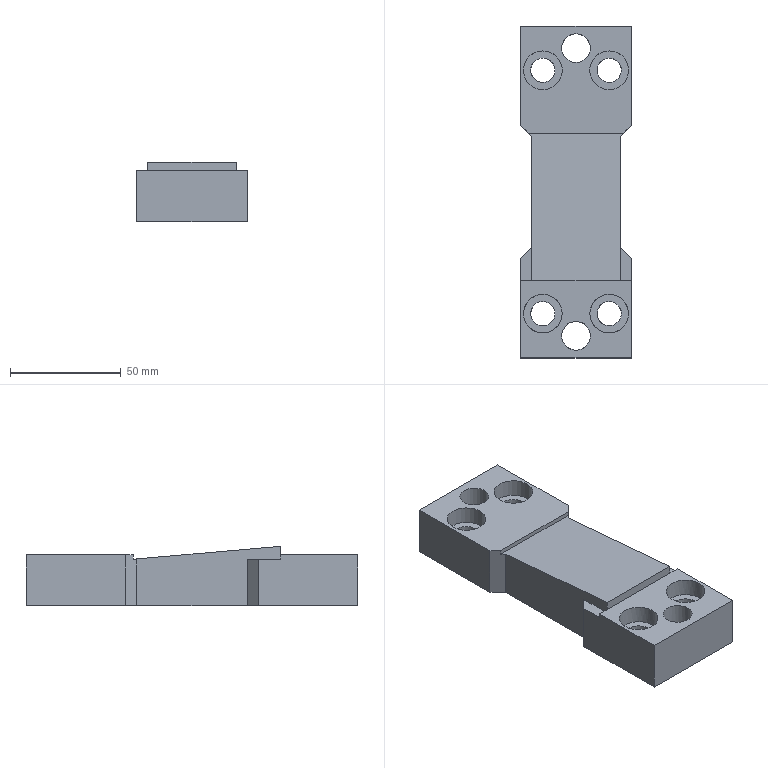Part | NX | features solid 2 | 1 solid | 36 faces | box 50 x 150 x 26.824 mm | volume 142519 mm3 | plane 26 | cylinder 10 | commonest cylinder face diameters 11 x4 17.5 x4 13 x2
STEP:
#1=CARTESIAN_POINT('',(-205.,-123.25,-57.));
#2=VERTEX_POINT('',#1);
#3=CARTESIAN_POINT('',(-205.,-132.,-57.));
#4=DIRECTION('',(0.,0.,1.));
#5=DIRECTION('',(0.,1.,0.));
#6=AXIS2_PLACEMENT_3D('',#3,#4,#5);
#7=CIRCLE('',#6,8.75);
#8=EDGE_CURVE('',#2,#2,#7,.T.);
#9=ORIENTED_EDGE('',*,*,#8,.F.);
#10=EDGE_LOOP('',(#9));
#11=FACE_BOUND('',#10,.T.);
#12=CARTESIAN_POINT('',(-220.,-115.5,-57.));
#13=VERTEX_POINT('',#12);
#14=CARTESIAN_POINT('',(-220.,-122.,-57.));
#15=DIRECTION('',(0.,0.,1.));
#16=DIRECTION('',(0.,1.,0.));
#17=AXIS2_PLACEMENT_3D('',#14,#15,#16);
#18=CIRCLE('',#17,6.5);
#19=EDGE_CURVE('',#13,#13,#18,.T.);
#20=ORIENTED_EDGE('',*,*,#19,.F.);
#21=EDGE_LOOP('',(#20));
#22=FACE_BOUND('',#21,.T.);
#23=CARTESIAN_POINT('',(-235.,-123.25,-57.));
#24=VERTEX_POINT('',#23);
#25=CARTESIAN_POINT('',(-235.,-132.,-57.));
#26=DIRECTION('',(0.,0.,1.));
#27=DIRECTION('',(0.,1.,0.));
#28=AXIS2_PLACEMENT_3D('',#25,#26,#27);
#29=CIRCLE('',#28,8.75);
#30=EDGE_CURVE('',#24,#24,#29,.T.);
#31=ORIENTED_EDGE('',*,*,#30,.F.);
#32=EDGE_LOOP('',(#31));
#33=FACE_BOUND('',#32,.T.);
#34=CARTESIAN_POINT('',(-241.57,-160.43,-57.));
#35=VERTEX_POINT('',#34);
#36=CARTESIAN_POINT('',(-198.43,-160.43,-57.));
#37=VERTEX_POINT('',#36);
#38=CARTESIAN_POINT('',(-240.,-160.43,-57.));
#39=DIRECTION('',(1.,0.,0.));
#40=VECTOR('',#39,1000.);
#41=LINE('',#38,#40);
#42=EDGE_CURVE('',#35,#37,#41,.T.);
#43=ORIENTED_EDGE('',*,*,#42,.T.);
#44=CARTESIAN_POINT('',(-195.,-157.,-57.));
#45=VERTEX_POINT('',#44);
#46=CARTESIAN_POINT('',(-200.,-162.,-57.));
#47=DIRECTION('',(0.7071,0.7071,0.));
#48=VECTOR('',#47,1000.);
#49=LINE('',#46,#48);
#50=EDGE_CURVE('',#37,#45,#49,.T.);
#51=ORIENTED_EDGE('',*,*,#50,.T.);
#52=CARTESIAN_POINT('',(-195.,-112.,-57.));
#53=VERTEX_POINT('',#52);
#54=CARTESIAN_POINT('',(-195.,-157.,-57.));
#55=DIRECTION('',(0.,1.,0.));
#56=VECTOR('',#55,1000.);
#57=LINE('',#54,#56);
#58=EDGE_CURVE('',#45,#53,#57,.T.);
#59=ORIENTED_EDGE('',*,*,#58,.T.);
#60=CARTESIAN_POINT('',(-245.,-112.,-57.));
#61=VERTEX_POINT('',#60);
#62=CARTESIAN_POINT('',(-245.,-112.,-57.));
#63=DIRECTION('',(1.,0.,0.));
#64=VECTOR('',#63,1000.);
#65=LINE('',#62,#64);
#66=EDGE_CURVE('',#61,#53,#65,.T.);
#67=ORIENTED_EDGE('',*,*,#66,.F.);
#68=CARTESIAN_POINT('',(-245.,-157.,-57.));
#69=VERTEX_POINT('',#68);
#70=CARTESIAN_POINT('',(-245.,-157.,-57.));
#71=DIRECTION('',(0.,1.,0.));
#72=VECTOR('',#71,1000.);
#73=LINE('',#70,#72);
#74=EDGE_CURVE('',#69,#61,#73,.T.);
#75=ORIENTED_EDGE('',*,*,#74,.F.);
#76=CARTESIAN_POINT('',(-240.,-162.,-57.));
#77=DIRECTION('',(-0.7071,0.7071,0.));
#78=VECTOR('',#77,1000.);
#79=LINE('',#76,#78);
#80=EDGE_CURVE('',#35,#69,#79,.T.);
#81=ORIENTED_EDGE('',*,*,#80,.F.);
#82=EDGE_LOOP('',(#43,#51,#59,#67,#75,#81));
#83=FACE_BOUND('',#82,.T.);
#84=CARTESIAN_POINT('',(-245.,-262.,-57.));
#85=DIRECTION('',(0.,0.,-1.));
#86=DIRECTION('',(-1.,0.,0.));
#87=AXIS2_PLACEMENT_3D('',#84,#85,#86);
#88=PLANE('',#87);
#89=ADVANCED_FACE('',(#11,#22,#33,#83),#88,.F.);
#90=CARTESIAN_POINT('',(-200.,-162.,-58.863));
#91=VERTEX_POINT('',#90);
#92=CARTESIAN_POINT('',(-200.,-162.,-80.));
#93=VERTEX_POINT('',#92);
#94=CARTESIAN_POINT('',(-200.,-162.,-59.));
#95=DIRECTION('',(0.,0.,-1.));
#96=VECTOR('',#95,1000.);
#97=LINE('',#94,#96);
#98=EDGE_CURVE('',#91,#93,#97,.T.);
#99=ORIENTED_EDGE('',*,*,#98,.F.);
#100=CARTESIAN_POINT('',(-200.,-227.,-53.176));
#101=VERTEX_POINT('',#100);
#102=CARTESIAN_POINT('',(-200.,-227.,-53.176));
#103=DIRECTION('',(0.,0.9962,-0.08716));
#104=VECTOR('',#103,1000.);
#105=LINE('',#102,#104);
#106=EDGE_CURVE('',#101,#91,#105,.T.);
#107=ORIENTED_EDGE('',*,*,#106,.F.);
#108=CARTESIAN_POINT('',(-200.,-227.,-57.));
#109=VERTEX_POINT('',#108);
#110=CARTESIAN_POINT('',(-200.,-227.,-53.176));
#111=DIRECTION('',(0.,0.,-1.));
#112=VECTOR('',#111,1000.);
#113=LINE('',#110,#112);
#114=EDGE_CURVE('',#101,#109,#113,.T.);
#115=ORIENTED_EDGE('',*,*,#114,.T.);
#116=CARTESIAN_POINT('',(-200.,-227.,-59.));
#117=VERTEX_POINT('',#116);
#118=CARTESIAN_POINT('',(-200.,-227.,-53.176));
#119=DIRECTION('',(0.,0.,-1.));
#120=VECTOR('',#119,1000.);
#121=LINE('',#118,#120);
#122=EDGE_CURVE('',#109,#117,#121,.T.);
#123=ORIENTED_EDGE('',*,*,#122,.T.);
#124=CARTESIAN_POINT('',(-200.,-212.,-59.));
#125=VERTEX_POINT('',#124);
#126=CARTESIAN_POINT('',(-200.,-160.43,-59.));
#127=DIRECTION('',(0.,-1.,0.));
#128=VECTOR('',#127,1000.);
#129=LINE('',#126,#128);
#130=EDGE_CURVE('',#125,#117,#129,.T.);
#131=ORIENTED_EDGE('',*,*,#130,.F.);
#132=CARTESIAN_POINT('',(-200.,-212.,-80.));
#133=VERTEX_POINT('',#132);
#134=CARTESIAN_POINT('',(-200.,-212.,-59.));
#135=DIRECTION('',(0.,0.,-1.));
#136=VECTOR('',#135,1000.);
#137=LINE('',#134,#136);
#138=EDGE_CURVE('',#125,#133,#137,.T.);
#139=ORIENTED_EDGE('',*,*,#138,.T.);
#140=CARTESIAN_POINT('',(-200.,-212.,-80.));
#141=DIRECTION('',(0.,1.,0.));
#142=VECTOR('',#141,1000.);
#143=LINE('',#140,#142);
#144=EDGE_CURVE('',#133,#93,#143,.T.);
#145=ORIENTED_EDGE('',*,*,#144,.T.);
#146=EDGE_LOOP('',(#99,#107,#115,#123,#131,#139,#145));
#147=FACE_BOUND('',#146,.T.);
#148=CARTESIAN_POINT('',(-200.,-212.,-59.));
#149=DIRECTION('',(-1.,0.,0.));
#150=DIRECTION('',(0.,-1.,0.));
#151=AXIS2_PLACEMENT_3D('',#148,#149,#150);
#152=PLANE('',#151);
#153=ADVANCED_FACE('',(#147),#152,.F.);
#154=CARTESIAN_POINT('',(-240.,-227.,-53.176));
#155=VERTEX_POINT('',#154);
#156=CARTESIAN_POINT('',(-240.,-227.,-57.));
#157=VERTEX_POINT('',#156);
#158=CARTESIAN_POINT('',(-240.,-227.,-53.176));
#159=DIRECTION('',(0.,0.,-1.));
#160=VECTOR('',#159,1000.);
#161=LINE('',#158,#160);
#162=EDGE_CURVE('',#155,#157,#161,.T.);
#163=ORIENTED_EDGE('',*,*,#162,.T.);
#164=CARTESIAN_POINT('',(-240.,-227.,-57.));
#165=DIRECTION('',(1.,0.,0.));
#166=VECTOR('',#165,1000.);
#167=LINE('',#164,#166);
#168=EDGE_CURVE('',#157,#109,#167,.T.);
#169=ORIENTED_EDGE('',*,*,#168,.T.);
#170=ORIENTED_EDGE('',*,*,#114,.F.);
#171=CARTESIAN_POINT('',(-240.,-227.,-53.176));
#172=DIRECTION('',(1.,0.,0.));
#173=VECTOR('',#172,1000.);
#174=LINE('',#171,#173);
#175=EDGE_CURVE('',#155,#101,#174,.T.);
#176=ORIENTED_EDGE('',*,*,#175,.F.);
#177=EDGE_LOOP('',(#163,#169,#170,#176));
#178=FACE_BOUND('',#177,.T.);
#179=CARTESIAN_POINT('',(-240.,-227.,-53.176));
#180=DIRECTION('',(0.,-1.,0.));
#181=DIRECTION('',(1.,0.,0.));
#182=AXIS2_PLACEMENT_3D('',#179,#180,#181);
#183=PLANE('',#182);
#184=ADVANCED_FACE('',(#178),#183,.T.);
#185=ORIENTED_EDGE('',*,*,#130,.T.);
#186=CARTESIAN_POINT('',(-195.,-227.,-59.));
#187=VERTEX_POINT('',#186);
#188=CARTESIAN_POINT('',(-245.,-227.,-59.));
#189=DIRECTION('',(1.,0.,0.));
#190=VECTOR('',#189,1000.);
#191=LINE('',#188,#190);
#192=EDGE_CURVE('',#117,#187,#191,.T.);
#193=ORIENTED_EDGE('',*,*,#192,.T.);
#194=CARTESIAN_POINT('',(-195.,-217.,-59.));
#195=VERTEX_POINT('',#194);
#196=CARTESIAN_POINT('',(-195.,-262.,-59.));
#197=DIRECTION('',(0.,1.,0.));
#198=VECTOR('',#197,1000.);
#199=LINE('',#196,#198);
#200=EDGE_CURVE('',#187,#195,#199,.T.);
#201=ORIENTED_EDGE('',*,*,#200,.T.);
#202=CARTESIAN_POINT('',(-200.,-212.,-59.));
#203=DIRECTION('',(0.7071,-0.7071,0.));
#204=VECTOR('',#203,1000.);
#205=LINE('',#202,#204);
#206=EDGE_CURVE('',#125,#195,#205,.T.);
#207=ORIENTED_EDGE('',*,*,#206,.F.);
#208=EDGE_LOOP('',(#185,#193,#201,#207));
#209=FACE_BOUND('',#208,.T.);
#210=CARTESIAN_POINT('',(-245.,-262.,-59.));
#211=DIRECTION('',(0.,0.,-1.));
#212=DIRECTION('',(-1.,0.,0.));
#213=AXIS2_PLACEMENT_3D('',#210,#211,#212);
#214=PLANE('',#213);
#215=ADVANCED_FACE('',(#209),#214,.F.);
#216=CARTESIAN_POINT('',(-245.,-227.,-59.));
#217=VERTEX_POINT('',#216);
#218=CARTESIAN_POINT('',(-240.,-227.,-59.));
#219=VERTEX_POINT('',#218);
#220=CARTESIAN_POINT('',(-245.,-227.,-59.));
#221=DIRECTION('',(1.,0.,0.));
#222=VECTOR('',#221,1000.);
#223=LINE('',#220,#222);
#224=EDGE_CURVE('',#217,#219,#223,.T.);
#225=ORIENTED_EDGE('',*,*,#224,.T.);
#226=CARTESIAN_POINT('',(-240.,-212.,-59.));
#227=VERTEX_POINT('',#226);
#228=CARTESIAN_POINT('',(-240.,-160.43,-59.));
#229=DIRECTION('',(0.,-1.,0.));
#230=VECTOR('',#229,1000.);
#231=LINE('',#228,#230);
#232=EDGE_CURVE('',#227,#219,#231,.T.);
#233=ORIENTED_EDGE('',*,*,#232,.F.);
#234=CARTESIAN_POINT('',(-245.,-217.,-59.));
#235=VERTEX_POINT('',#234);
#236=CARTESIAN_POINT('',(-245.,-217.,-59.));
#237=DIRECTION('',(0.7071,0.7071,0.));
#238=VECTOR('',#237,1000.);
#239=LINE('',#236,#238);
#240=EDGE_CURVE('',#235,#227,#239,.T.);
#241=ORIENTED_EDGE('',*,*,#240,.F.);
#242=CARTESIAN_POINT('',(-245.,-262.,-59.));
#243=DIRECTION('',(0.,1.,0.));
#244=VECTOR('',#243,1000.);
#245=LINE('',#242,#244);
#246=EDGE_CURVE('',#217,#235,#245,.T.);
#247=ORIENTED_EDGE('',*,*,#246,.F.);
#248=EDGE_LOOP('',(#225,#233,#241,#247));
#249=FACE_BOUND('',#248,.T.);
#250=CARTESIAN_POINT('',(-245.,-262.,-59.));
#251=DIRECTION('',(0.,0.,-1.));
#252=DIRECTION('',(-1.,0.,0.));
#253=AXIS2_PLACEMENT_3D('',#250,#251,#252);
#254=PLANE('',#253);
#255=ADVANCED_FACE('',(#249),#254,.F.);
#256=ORIENTED_EDGE('',*,*,#192,.F.);
#257=ORIENTED_EDGE('',*,*,#122,.F.);
#258=CARTESIAN_POINT('',(-195.,-227.,-57.));
#259=VERTEX_POINT('',#258);
#260=CARTESIAN_POINT('',(-245.,-227.,-57.));
#261=DIRECTION('',(1.,0.,0.));
#262=VECTOR('',#261,1000.);
#263=LINE('',#260,#262);
#264=EDGE_CURVE('',#109,#259,#263,.T.);
#265=ORIENTED_EDGE('',*,*,#264,.T.);
#266=CARTESIAN_POINT('',(-195.,-227.,-59.));
#267=DIRECTION('',(0.,0.,-1.));
#268=VECTOR('',#267,1000.);
#269=LINE('',#266,#268);
#270=EDGE_CURVE('',#259,#187,#269,.T.);
#271=ORIENTED_EDGE('',*,*,#270,.T.);
#272=EDGE_LOOP('',(#256,#257,#265,#271));
#273=FACE_BOUND('',#272,.T.);
#274=CARTESIAN_POINT('',(-245.,-227.,-40.44));
#275=DIRECTION('',(0.,1.,0.));
#276=DIRECTION('',(-1.,0.,0.));
#277=AXIS2_PLACEMENT_3D('',#274,#275,#276);
#278=PLANE('',#277);
#279=ADVANCED_FACE('',(#273),#278,.T.);
#280=CARTESIAN_POINT('',(-205.,-126.5,-80.));
#281=VERTEX_POINT('',#280);
#282=CARTESIAN_POINT('',(-205.,-132.,-80.));
#283=DIRECTION('',(0.,0.,1.));
#284=DIRECTION('',(0.,1.,0.));
#285=AXIS2_PLACEMENT_3D('',#282,#283,#284);
#286=CIRCLE('',#285,5.5);
#287=EDGE_CURVE('',#281,#281,#286,.T.);
#288=ORIENTED_EDGE('',*,*,#287,.F.);
#289=EDGE_LOOP('',(#288));
#290=FACE_BOUND('',#289,.T.);
#291=CARTESIAN_POINT('',(-199.5,-132.,-65.));
#292=VERTEX_POINT('',#291);
#293=CARTESIAN_POINT('',(-205.,-132.,-65.));
#294=DIRECTION('',(0.,0.,1.));
#295=DIRECTION('',(1.,0.,0.));
#296=AXIS2_PLACEMENT_3D('',#293,#294,#295);
#297=CIRCLE('',#296,5.5);
#298=EDGE_CURVE('',#292,#292,#297,.T.);
#299=ORIENTED_EDGE('',*,*,#298,.T.);
#300=EDGE_LOOP('',(#299));
#301=FACE_BOUND('',#300,.T.);
#302=CARTESIAN_POINT('',(-205.,-132.,-59.));
#303=DIRECTION('',(0.,0.,-1.));
#304=DIRECTION('',(-1.,0.,0.));
#305=AXIS2_PLACEMENT_3D('',#302,#303,#304);
#306=CYLINDRICAL_SURFACE('',#305,5.5);
#307=ADVANCED_FACE('',(#290,#301),#306,.F.);
#308=CARTESIAN_POINT('',(-235.,-126.5,-80.));
#309=VERTEX_POINT('',#308);
#310=CARTESIAN_POINT('',(-235.,-132.,-80.));
#311=DIRECTION('',(0.,0.,1.));
#312=DIRECTION('',(0.,1.,0.));
#313=AXIS2_PLACEMENT_3D('',#310,#311,#312);
#314=CIRCLE('',#313,5.5);
#315=EDGE_CURVE('',#309,#309,#314,.T.);
#316=ORIENTED_EDGE('',*,*,#315,.F.);
#317=EDGE_LOOP('',(#316));
#318=FACE_BOUND('',#317,.T.);
#319=CARTESIAN_POINT('',(-229.5,-132.,-65.));
#320=VERTEX_POINT('',#319);
#321=CARTESIAN_POINT('',(-235.,-132.,-65.));
#322=DIRECTION('',(0.,0.,1.));
#323=DIRECTION('',(1.,0.,0.));
#324=AXIS2_PLACEMENT_3D('',#321,#322,#323);
#325=CIRCLE('',#324,5.5);
#326=EDGE_CURVE('',#320,#320,#325,.T.);
#327=ORIENTED_EDGE('',*,*,#326,.T.);
#328=EDGE_LOOP('',(#327));
#329=FACE_BOUND('',#328,.T.);
#330=CARTESIAN_POINT('',(-235.,-132.,-59.));
#331=DIRECTION('',(0.,0.,-1.));
#332=DIRECTION('',(-1.,0.,0.));
#333=AXIS2_PLACEMENT_3D('',#330,#331,#332);
#334=CYLINDRICAL_SURFACE('',#333,5.5);
#335=ADVANCED_FACE('',(#318,#329),#334,.F.);
#336=CARTESIAN_POINT('',(-195.,-262.,-80.));
#337=VERTEX_POINT('',#336);
#338=CARTESIAN_POINT('',(-195.,-217.,-80.));
#339=VERTEX_POINT('',#338);
#340=CARTESIAN_POINT('',(-195.,-262.,-80.));
#341=DIRECTION('',(0.,1.,0.));
#342=VECTOR('',#341,1000.);
#343=LINE('',#340,#342);
#344=EDGE_CURVE('',#337,#339,#343,.T.);
#345=ORIENTED_EDGE('',*,*,#344,.F.);
#346=CARTESIAN_POINT('',(-245.,-262.,-80.));
#347=VERTEX_POINT('',#346);
#348=CARTESIAN_POINT('',(-195.,-262.,-80.));
#349=DIRECTION('',(-1.,0.,0.));
#350=VECTOR('',#349,1000.);
#351=LINE('',#348,#350);
#352=EDGE_CURVE('',#337,#347,#351,.T.);
#353=ORIENTED_EDGE('',*,*,#352,.T.);
#354=CARTESIAN_POINT('',(-245.,-217.,-80.));
#355=VERTEX_POINT('',#354);
#356=CARTESIAN_POINT('',(-245.,-262.,-80.));
#357=DIRECTION('',(0.,1.,0.));
#358=VECTOR('',#357,1000.);
#359=LINE('',#356,#358);
#360=EDGE_CURVE('',#347,#355,#359,.T.);
#361=ORIENTED_EDGE('',*,*,#360,.T.);
#362=CARTESIAN_POINT('',(-240.,-212.,-80.));
#363=VERTEX_POINT('',#362);
#364=CARTESIAN_POINT('',(-245.,-217.,-80.));
#365=DIRECTION('',(0.7071,0.7071,0.));
#366=VECTOR('',#365,1000.);
#367=LINE('',#364,#366);
#368=EDGE_CURVE('',#355,#363,#367,.T.);
#369=ORIENTED_EDGE('',*,*,#368,.T.);
#370=CARTESIAN_POINT('',(-240.,-162.,-80.));
#371=VERTEX_POINT('',#370);
#372=CARTESIAN_POINT('',(-240.,-212.,-80.));
#373=DIRECTION('',(0.,1.,0.));
#374=VECTOR('',#373,1000.);
#375=LINE('',#372,#374);
#376=EDGE_CURVE('',#363,#371,#375,.T.);
#377=ORIENTED_EDGE('',*,*,#376,.T.);
#378=CARTESIAN_POINT('',(-245.,-157.,-80.));
#379=VERTEX_POINT('',#378);
#380=CARTESIAN_POINT('',(-240.,-162.,-80.));
#381=DIRECTION('',(-0.7071,0.7071,0.));
#382=VECTOR('',#381,1000.);
#383=LINE('',#380,#382);
#384=EDGE_CURVE('',#371,#379,#383,.T.);
#385=ORIENTED_EDGE('',*,*,#384,.T.);
#386=CARTESIAN_POINT('',(-245.,-112.,-80.));
#387=VERTEX_POINT('',#386);
#388=CARTESIAN_POINT('',(-245.,-157.,-80.));
#389=DIRECTION('',(0.,1.,0.));
#390=VECTOR('',#389,1000.);
#391=LINE('',#388,#390);
#392=EDGE_CURVE('',#379,#387,#391,.T.);
#393=ORIENTED_EDGE('',*,*,#392,.T.);
#394=CARTESIAN_POINT('',(-195.,-112.,-80.));
#395=VERTEX_POINT('',#394);
#396=CARTESIAN_POINT('',(-245.,-112.,-80.));
#397=DIRECTION('',(1.,0.,0.));
#398=VECTOR('',#397,1000.);
#399=LINE('',#396,#398);
#400=EDGE_CURVE('',#387,#395,#399,.T.);
#401=ORIENTED_EDGE('',*,*,#400,.T.);
#402=CARTESIAN_POINT('',(-195.,-157.,-80.));
#403=VERTEX_POINT('',#402);
#404=CARTESIAN_POINT('',(-195.,-157.,-80.));
#405=DIRECTION('',(0.,1.,0.));
#406=VECTOR('',#405,1000.);
#407=LINE('',#404,#406);
#408=EDGE_CURVE('',#403,#395,#407,.T.);
#409=ORIENTED_EDGE('',*,*,#408,.F.);
#410=CARTESIAN_POINT('',(-200.,-162.,-80.));
#411=DIRECTION('',(0.7071,0.7071,0.));
#412=VECTOR('',#411,1000.);
#413=LINE('',#410,#412);
#414=EDGE_CURVE('',#93,#403,#413,.T.);
#415=ORIENTED_EDGE('',*,*,#414,.F.);
#416=ORIENTED_EDGE('',*,*,#144,.F.);
#417=CARTESIAN_POINT('',(-200.,-212.,-80.));
#418=DIRECTION('',(0.7071,-0.7071,0.));
#419=VECTOR('',#418,1000.);
#420=LINE('',#417,#419);
#421=EDGE_CURVE('',#133,#339,#420,.T.);
#422=ORIENTED_EDGE('',*,*,#421,.T.);
#423=EDGE_LOOP('',(#345,#353,#361,#369,#377,#385,#393,#401,#409,#415,#416,#422));
#424=FACE_BOUND('',#423,.T.);
#425=ORIENTED_EDGE('',*,*,#287,.T.);
#426=EDGE_LOOP('',(#425));
#427=FACE_BOUND('',#426,.T.);
#428=ORIENTED_EDGE('',*,*,#315,.T.);
#429=EDGE_LOOP('',(#428));
#430=FACE_BOUND('',#429,.T.);
#431=CARTESIAN_POINT('',(-220.,-115.5,-80.));
#432=VERTEX_POINT('',#431);
#433=CARTESIAN_POINT('',(-220.,-122.,-80.));
#434=DIRECTION('',(0.,0.,1.));
#435=DIRECTION('',(0.,1.,0.));
#436=AXIS2_PLACEMENT_3D('',#433,#434,#435);
#437=CIRCLE('',#436,6.5);
#438=EDGE_CURVE('',#432,#432,#437,.T.);
#439=ORIENTED_EDGE('',*,*,#438,.T.);
#440=EDGE_LOOP('',(#439));
#441=FACE_BOUND('',#440,.T.);
#442=CARTESIAN_POINT('',(-205.,-236.5,-80.));
#443=VERTEX_POINT('',#442);
#444=CARTESIAN_POINT('',(-205.,-242.,-80.));
#445=DIRECTION('',(0.,0.,1.));
#446=DIRECTION('',(0.,1.,0.));
#447=AXIS2_PLACEMENT_3D('',#444,#445,#446);
#448=CIRCLE('',#447,5.5);
#449=EDGE_CURVE('',#443,#443,#448,.T.);
#450=ORIENTED_EDGE('',*,*,#449,.T.);
#451=EDGE_LOOP('',(#450));
#452=FACE_BOUND('',#451,.T.);
#453=CARTESIAN_POINT('',(-235.,-236.5,-80.));
#454=VERTEX_POINT('',#453);
#455=CARTESIAN_POINT('',(-235.,-242.,-80.));
#456=DIRECTION('',(0.,0.,1.));
#457=DIRECTION('',(0.,1.,0.));
#458=AXIS2_PLACEMENT_3D('',#455,#456,#457);
#459=CIRCLE('',#458,5.5);
#460=EDGE_CURVE('',#454,#454,#459,.T.);
#461=ORIENTED_EDGE('',*,*,#460,.T.);
#462=EDGE_LOOP('',(#461));
#463=FACE_BOUND('',#462,.T.);
#464=CARTESIAN_POINT('',(-220.,-245.5,-80.));
#465=VERTEX_POINT('',#464);
#466=CARTESIAN_POINT('',(-220.,-252.,-80.));
#467=DIRECTION('',(0.,0.,1.));
#468=DIRECTION('',(0.,1.,0.));
#469=AXIS2_PLACEMENT_3D('',#466,#467,#468);
#470=CIRCLE('',#469,6.5);
#471=EDGE_CURVE('',#465,#465,#470,.T.);
#472=ORIENTED_EDGE('',*,*,#471,.T.);
#473=EDGE_LOOP('',(#472));
#474=FACE_BOUND('',#473,.T.);
#475=CARTESIAN_POINT('',(-245.,-262.,-80.));
#476=DIRECTION('',(0.,0.,-1.));
#477=DIRECTION('',(-1.,0.,0.));
#478=AXIS2_PLACEMENT_3D('',#475,#476,#477);
#479=PLANE('',#478);
#480=ADVANCED_FACE('',(#424,#427,#430,#441,#452,#463,#474),#479,.T.);
#481=ORIENTED_EDGE('',*,*,#360,.F.);
#482=CARTESIAN_POINT('',(-245.,-262.,-57.));
#483=VERTEX_POINT('',#482);
#484=CARTESIAN_POINT('',(-245.,-262.,-59.));
#485=DIRECTION('',(0.,0.,-1.));
#486=VECTOR('',#485,1000.);
#487=LINE('',#484,#486);
#488=EDGE_CURVE('',#483,#347,#487,.T.);
#489=ORIENTED_EDGE('',*,*,#488,.F.);
#490=CARTESIAN_POINT('',(-245.,-227.,-57.));
#491=VERTEX_POINT('',#490);
#492=CARTESIAN_POINT('',(-245.,-262.,-57.));
#493=DIRECTION('',(0.,1.,0.));
#494=VECTOR('',#493,1000.);
#495=LINE('',#492,#494);
#496=EDGE_CURVE('',#483,#491,#495,.T.);
#497=ORIENTED_EDGE('',*,*,#496,.T.);
#498=CARTESIAN_POINT('',(-245.,-227.,-59.));
#499=DIRECTION('',(0.,0.,-1.));
#500=VECTOR('',#499,1000.);
#501=LINE('',#498,#500);
#502=EDGE_CURVE('',#491,#217,#501,.T.);
#503=ORIENTED_EDGE('',*,*,#502,.T.);
#504=ORIENTED_EDGE('',*,*,#246,.T.);
#505=CARTESIAN_POINT('',(-245.,-217.,-59.));
#506=DIRECTION('',(0.,0.,-1.));
#507=VECTOR('',#506,1000.);
#508=LINE('',#505,#507);
#509=EDGE_CURVE('',#235,#355,#508,.T.);
#510=ORIENTED_EDGE('',*,*,#509,.T.);
#511=EDGE_LOOP('',(#481,#489,#497,#503,#504,#510));
#512=FACE_BOUND('',#511,.T.);
#513=CARTESIAN_POINT('',(-245.,-262.,-59.));
#514=DIRECTION('',(-1.,0.,0.));
#515=DIRECTION('',(0.,-1.,0.));
#516=AXIS2_PLACEMENT_3D('',#513,#514,#515);
#517=PLANE('',#516);
#518=ADVANCED_FACE('',(#512),#517,.T.);
#519=ORIENTED_EDGE('',*,*,#368,.F.);
#520=ORIENTED_EDGE('',*,*,#509,.F.);
#521=ORIENTED_EDGE('',*,*,#240,.T.);
#522=CARTESIAN_POINT('',(-240.,-212.,-59.));
#523=DIRECTION('',(0.,0.,-1.));
#524=VECTOR('',#523,1000.);
#525=LINE('',#522,#524);
#526=EDGE_CURVE('',#227,#363,#525,.T.);
#527=ORIENTED_EDGE('',*,*,#526,.T.);
#528=EDGE_LOOP('',(#519,#520,#521,#527));
#529=FACE_BOUND('',#528,.T.);
#530=CARTESIAN_POINT('',(-245.,-217.,-59.));
#531=DIRECTION('',(-0.7071,0.7071,0.));
#532=DIRECTION('',(-0.7071,-0.7071,0.));
#533=AXIS2_PLACEMENT_3D('',#530,#531,#532);
#534=PLANE('',#533);
#535=ADVANCED_FACE('',(#529),#534,.T.);
#536=CARTESIAN_POINT('',(-240.,-162.,-58.863));
#537=VERTEX_POINT('',#536);
#538=CARTESIAN_POINT('',(-240.,-227.,-53.176));
#539=DIRECTION('',(0.,0.9962,-0.08716));
#540=VECTOR('',#539,1000.);
#541=LINE('',#538,#540);
#542=EDGE_CURVE('',#155,#537,#541,.T.);
#543=ORIENTED_EDGE('',*,*,#542,.T.);
#544=CARTESIAN_POINT('',(-240.,-162.,-59.));
#545=DIRECTION('',(0.,0.,-1.));
#546=VECTOR('',#545,1000.);
#547=LINE('',#544,#546);
#548=EDGE_CURVE('',#537,#371,#547,.T.);
#549=ORIENTED_EDGE('',*,*,#548,.T.);
#550=ORIENTED_EDGE('',*,*,#376,.F.);
#551=ORIENTED_EDGE('',*,*,#526,.F.);
#552=ORIENTED_EDGE('',*,*,#232,.T.);
#553=CARTESIAN_POINT('',(-240.,-227.,-53.176));
#554=DIRECTION('',(0.,0.,-1.));
#555=VECTOR('',#554,1000.);
#556=LINE('',#553,#555);
#557=EDGE_CURVE('',#157,#219,#556,.T.);
#558=ORIENTED_EDGE('',*,*,#557,.F.);
#559=ORIENTED_EDGE('',*,*,#162,.F.);
#560=EDGE_LOOP('',(#543,#549,#550,#551,#552,#558,#559));
#561=FACE_BOUND('',#560,.T.);
#562=CARTESIAN_POINT('',(-240.,-212.,-59.));
#563=DIRECTION('',(-1.,0.,0.));
#564=DIRECTION('',(0.,-1.,0.));
#565=AXIS2_PLACEMENT_3D('',#562,#563,#564);
#566=PLANE('',#565);
#567=ADVANCED_FACE('',(#561),#566,.T.);
#568=CARTESIAN_POINT('',(-241.57,-160.43,-59.));
#569=VERTEX_POINT('',#568);
#570=CARTESIAN_POINT('',(-240.006,-161.994,-58.863));
#571=DIRECTION('',(0.7058,-0.7058,0.06175));
#572=VECTOR('',#571,1000.);
#573=LINE('',#570,#572);
#574=EDGE_CURVE('',#569,#537,#573,.T.);
#575=ORIENTED_EDGE('',*,*,#574,.F.);
#576=CARTESIAN_POINT('',(-241.57,-160.43,-59.));
#577=DIRECTION('',(0.,0.,1.));
#578=VECTOR('',#577,1000.);
#579=LINE('',#576,#578);
#580=EDGE_CURVE('',#569,#35,#579,.T.);
#581=ORIENTED_EDGE('',*,*,#580,.T.);
#582=ORIENTED_EDGE('',*,*,#80,.T.);
#583=CARTESIAN_POINT('',(-245.,-157.,-59.));
#584=DIRECTION('',(0.,0.,-1.));
#585=VECTOR('',#584,1000.);
#586=LINE('',#583,#585);
#587=EDGE_CURVE('',#69,#379,#586,.T.);
#588=ORIENTED_EDGE('',*,*,#587,.T.);
#589=ORIENTED_EDGE('',*,*,#384,.F.);
#590=ORIENTED_EDGE('',*,*,#548,.F.);
#591=EDGE_LOOP('',(#575,#581,#582,#588,#589,#590));
#592=FACE_BOUND('',#591,.T.);
#593=CARTESIAN_POINT('',(-240.,-162.,-59.));
#594=DIRECTION('',(-0.7071,-0.7071,0.));
#595=DIRECTION('',(0.7071,-0.7071,0.));
#596=AXIS2_PLACEMENT_3D('',#593,#594,#595);
#597=PLANE('',#596);
#598=ADVANCED_FACE('',(#592),#597,.T.);
#599=ORIENTED_EDGE('',*,*,#392,.F.);
#600=ORIENTED_EDGE('',*,*,#587,.F.);
#601=ORIENTED_EDGE('',*,*,#74,.T.);
#602=CARTESIAN_POINT('',(-245.,-112.,-59.));
#603=DIRECTION('',(0.,0.,-1.));
#604=VECTOR('',#603,1000.);
#605=LINE('',#602,#604);
#606=EDGE_CURVE('',#61,#387,#605,.T.);
#607=ORIENTED_EDGE('',*,*,#606,.T.);
#608=EDGE_LOOP('',(#599,#600,#601,#607));
#609=FACE_BOUND('',#608,.T.);
#610=CARTESIAN_POINT('',(-245.,-157.,-59.));
#611=DIRECTION('',(-1.,0.,0.));
#612=DIRECTION('',(0.,-1.,0.));
#613=AXIS2_PLACEMENT_3D('',#610,#611,#612);
#614=PLANE('',#613);
#615=ADVANCED_FACE('',(#609),#614,.T.);
#616=ORIENTED_EDGE('',*,*,#400,.F.);
#617=ORIENTED_EDGE('',*,*,#606,.F.);
#618=ORIENTED_EDGE('',*,*,#66,.T.);
#619=CARTESIAN_POINT('',(-195.,-112.,-59.));
#620=DIRECTION('',(0.,0.,-1.));
#621=VECTOR('',#620,1000.);
#622=LINE('',#619,#621);
#623=EDGE_CURVE('',#53,#395,#622,.T.);
#624=ORIENTED_EDGE('',*,*,#623,.T.);
#625=EDGE_LOOP('',(#616,#617,#618,#624));
#626=FACE_BOUND('',#625,.T.);
#627=CARTESIAN_POINT('',(-245.,-112.,-59.));
#628=DIRECTION('',(0.,1.,0.));
#629=DIRECTION('',(-1.,0.,0.));
#630=AXIS2_PLACEMENT_3D('',#627,#628,#629);
#631=PLANE('',#630);
#632=ADVANCED_FACE('',(#626),#631,.T.);
#633=ORIENTED_EDGE('',*,*,#408,.T.);
#634=ORIENTED_EDGE('',*,*,#623,.F.);
#635=ORIENTED_EDGE('',*,*,#58,.F.);
#636=CARTESIAN_POINT('',(-195.,-157.,-59.));
#637=DIRECTION('',(0.,0.,-1.));
#638=VECTOR('',#637,1000.);
#639=LINE('',#636,#638);
#640=EDGE_CURVE('',#45,#403,#639,.T.);
#641=ORIENTED_EDGE('',*,*,#640,.T.);
#642=EDGE_LOOP('',(#633,#634,#635,#641));
#643=FACE_BOUND('',#642,.T.);
#644=CARTESIAN_POINT('',(-195.,-157.,-59.));
#645=DIRECTION('',(-1.,0.,0.));
#646=DIRECTION('',(0.,-1.,0.));
#647=AXIS2_PLACEMENT_3D('',#644,#645,#646);
#648=PLANE('',#647);
#649=ADVANCED_FACE('',(#643),#648,.F.);
#650=ORIENTED_EDGE('',*,*,#50,.F.);
#651=CARTESIAN_POINT('',(-198.43,-160.43,-59.));
#652=VERTEX_POINT('',#651);
#653=CARTESIAN_POINT('',(-198.43,-160.43,-59.));
#654=DIRECTION('',(0.,0.,-1.));
#655=VECTOR('',#654,1000.);
#656=LINE('',#653,#655);
#657=EDGE_CURVE('',#37,#652,#656,.T.);
#658=ORIENTED_EDGE('',*,*,#657,.T.);
#659=CARTESIAN_POINT('',(-199.994,-161.994,-58.863));
#660=DIRECTION('',(0.7058,0.7058,-0.06175));
#661=VECTOR('',#660,1000.);
#662=LINE('',#659,#661);
#663=EDGE_CURVE('',#91,#652,#662,.T.);
#664=ORIENTED_EDGE('',*,*,#663,.F.);
#665=ORIENTED_EDGE('',*,*,#98,.T.);
#666=ORIENTED_EDGE('',*,*,#414,.T.);
#667=ORIENTED_EDGE('',*,*,#640,.F.);
#668=EDGE_LOOP('',(#650,#658,#664,#665,#666,#667));
#669=FACE_BOUND('',#668,.T.);
#670=CARTESIAN_POINT('',(-200.,-162.,-59.));
#671=DIRECTION('',(-0.7071,0.7071,0.));
#672=DIRECTION('',(-0.7071,-0.7071,0.));
#673=AXIS2_PLACEMENT_3D('',#670,#671,#672);
#674=PLANE('',#673);
#675=ADVANCED_FACE('',(#669),#674,.F.);
#676=ORIENTED_EDGE('',*,*,#421,.F.);
#677=ORIENTED_EDGE('',*,*,#138,.F.);
#678=ORIENTED_EDGE('',*,*,#206,.T.);
#679=CARTESIAN_POINT('',(-195.,-217.,-59.));
#680=DIRECTION('',(0.,0.,-1.));
#681=VECTOR('',#680,1000.);
#682=LINE('',#679,#681);
#683=EDGE_CURVE('',#195,#339,#682,.T.);
#684=ORIENTED_EDGE('',*,*,#683,.T.);
#685=EDGE_LOOP('',(#676,#677,#678,#684));
#686=FACE_BOUND('',#685,.T.);
#687=CARTESIAN_POINT('',(-200.,-212.,-59.));
#688=DIRECTION('',(0.7071,0.7071,0.));
#689=DIRECTION('',(-0.7071,0.7071,0.));
#690=AXIS2_PLACEMENT_3D('',#687,#688,#689);
#691=PLANE('',#690);
#692=ADVANCED_FACE('',(#686),#691,.T.);
#693=ORIENTED_EDGE('',*,*,#200,.F.);
#694=ORIENTED_EDGE('',*,*,#270,.F.);
#695=CARTESIAN_POINT('',(-195.,-262.,-57.));
#696=VERTEX_POINT('',#695);
#697=CARTESIAN_POINT('',(-195.,-262.,-57.));
#698=DIRECTION('',(0.,1.,0.));
#699=VECTOR('',#698,1000.);
#700=LINE('',#697,#699);
#701=EDGE_CURVE('',#696,#259,#700,.T.);
#702=ORIENTED_EDGE('',*,*,#701,.F.);
#703=CARTESIAN_POINT('',(-195.,-262.,-59.));
#704=DIRECTION('',(0.,0.,-1.));
#705=VECTOR('',#704,1000.);
#706=LINE('',#703,#705);
#707=EDGE_CURVE('',#696,#337,#706,.T.);
#708=ORIENTED_EDGE('',*,*,#707,.T.);
#709=ORIENTED_EDGE('',*,*,#344,.T.);
#710=ORIENTED_EDGE('',*,*,#683,.F.);
#711=EDGE_LOOP('',(#693,#694,#702,#708,#709,#710));
#712=FACE_BOUND('',#711,.T.);
#713=CARTESIAN_POINT('',(-195.,-262.,-59.));
#714=DIRECTION('',(-1.,0.,0.));
#715=DIRECTION('',(0.,-1.,0.));
#716=AXIS2_PLACEMENT_3D('',#713,#714,#715);
#717=PLANE('',#716);
#718=ADVANCED_FACE('',(#712),#717,.F.);
#719=ORIENTED_EDGE('',*,*,#438,.F.);
#720=EDGE_LOOP('',(#719));
#721=FACE_BOUND('',#720,.T.);
#722=ORIENTED_EDGE('',*,*,#19,.T.);
#723=EDGE_LOOP('',(#722));
#724=FACE_BOUND('',#723,.T.);
#725=CARTESIAN_POINT('',(-220.,-122.,-59.));
#726=DIRECTION('',(0.,0.,-1.));
#727=DIRECTION('',(-1.,0.,0.));
#728=AXIS2_PLACEMENT_3D('',#725,#726,#727);
#729=CYLINDRICAL_SURFACE('',#728,6.5);
#730=ADVANCED_FACE('',(#721,#724),#729,.F.);
#731=CARTESIAN_POINT('',(-235.,-123.25,-65.));
#732=VERTEX_POINT('',#731);
#733=CARTESIAN_POINT('',(-235.,-132.,-65.));
#734=DIRECTION('',(0.,0.,1.));
#735=DIRECTION('',(0.,1.,0.));
#736=AXIS2_PLACEMENT_3D('',#733,#734,#735);
#737=CIRCLE('',#736,8.75);
#738=EDGE_CURVE('',#732,#732,#737,.T.);
#739=ORIENTED_EDGE('',*,*,#738,.F.);
#740=EDGE_LOOP('',(#739));
#741=FACE_BOUND('',#740,.T.);
#742=ORIENTED_EDGE('',*,*,#30,.T.);
#743=EDGE_LOOP('',(#742));
#744=FACE_BOUND('',#743,.T.);
#745=CARTESIAN_POINT('',(-235.,-132.,-59.));
#746=DIRECTION('',(0.,0.,-1.));
#747=DIRECTION('',(-1.,0.,0.));
#748=AXIS2_PLACEMENT_3D('',#745,#746,#747);
#749=CYLINDRICAL_SURFACE('',#748,8.75);
#750=ADVANCED_FACE('',(#741,#744),#749,.F.);
#751=ORIENTED_EDGE('',*,*,#326,.F.);
#752=EDGE_LOOP('',(#751));
#753=FACE_BOUND('',#752,.T.);
#754=ORIENTED_EDGE('',*,*,#738,.T.);
#755=EDGE_LOOP('',(#754));
#756=FACE_BOUND('',#755,.T.);
#757=CARTESIAN_POINT('',(-235.,-132.,-65.));
#758=DIRECTION('',(0.,0.,1.));
#759=DIRECTION('',(1.,0.,0.));
#760=AXIS2_PLACEMENT_3D('',#757,#758,#759);
#761=PLANE('',#760);
#762=ADVANCED_FACE('',(#753,#756),#761,.T.);
#763=CARTESIAN_POINT('',(-205.,-123.25,-65.));
#764=VERTEX_POINT('',#763);
#765=CARTESIAN_POINT('',(-205.,-132.,-65.));
#766=DIRECTION('',(0.,0.,1.));
#767=DIRECTION('',(0.,1.,0.));
#768=AXIS2_PLACEMENT_3D('',#765,#766,#767);
#769=CIRCLE('',#768,8.75);
#770=EDGE_CURVE('',#764,#764,#769,.T.);
#771=ORIENTED_EDGE('',*,*,#770,.F.);
#772=EDGE_LOOP('',(#771));
#773=FACE_BOUND('',#772,.T.);
#774=ORIENTED_EDGE('',*,*,#8,.T.);
#775=EDGE_LOOP('',(#774));
#776=FACE_BOUND('',#775,.T.);
#777=CARTESIAN_POINT('',(-205.,-132.,-59.));
#778=DIRECTION('',(0.,0.,-1.));
#779=DIRECTION('',(-1.,0.,0.));
#780=AXIS2_PLACEMENT_3D('',#777,#778,#779);
#781=CYLINDRICAL_SURFACE('',#780,8.75);
#782=ADVANCED_FACE('',(#773,#776),#781,.F.);
#783=ORIENTED_EDGE('',*,*,#298,.F.);
#784=EDGE_LOOP('',(#783));
#785=FACE_BOUND('',#784,.T.);
#786=ORIENTED_EDGE('',*,*,#770,.T.);
#787=EDGE_LOOP('',(#786));
#788=FACE_BOUND('',#787,.T.);
#789=CARTESIAN_POINT('',(-205.,-132.,-65.));
#790=DIRECTION('',(0.,0.,1.));
#791=DIRECTION('',(1.,0.,0.));
#792=AXIS2_PLACEMENT_3D('',#789,#790,#791);
#793=PLANE('',#792);
#794=ADVANCED_FACE('',(#785,#788),#793,.T.);
#795=ORIENTED_EDGE('',*,*,#557,.T.);
#796=ORIENTED_EDGE('',*,*,#224,.F.);
#797=ORIENTED_EDGE('',*,*,#502,.F.);
#798=CARTESIAN_POINT('',(-245.,-227.,-57.));
#799=DIRECTION('',(1.,0.,0.));
#800=VECTOR('',#799,1000.);
#801=LINE('',#798,#800);
#802=EDGE_CURVE('',#491,#157,#801,.T.);
#803=ORIENTED_EDGE('',*,*,#802,.T.);
#804=EDGE_LOOP('',(#795,#796,#797,#803));
#805=FACE_BOUND('',#804,.T.);
#806=CARTESIAN_POINT('',(-245.,-227.,-40.44));
#807=DIRECTION('',(0.,1.,0.));
#808=DIRECTION('',(-1.,0.,0.));
#809=AXIS2_PLACEMENT_3D('',#806,#807,#808);
#810=PLANE('',#809);
#811=ADVANCED_FACE('',(#805),#810,.T.);
#812=CARTESIAN_POINT('',(-229.5,-242.,-65.));
#813=VERTEX_POINT('',#812);
#814=CARTESIAN_POINT('',(-235.,-242.,-65.));
#815=DIRECTION('',(0.,0.,1.));
#816=DIRECTION('',(1.,0.,0.));
#817=AXIS2_PLACEMENT_3D('',#814,#815,#816);
#818=CIRCLE('',#817,5.5);
#819=EDGE_CURVE('',#813,#813,#818,.T.);
#820=ORIENTED_EDGE('',*,*,#819,.F.);
#821=EDGE_LOOP('',(#820));
#822=FACE_BOUND('',#821,.T.);
#823=CARTESIAN_POINT('',(-235.,-233.25,-65.));
#824=VERTEX_POINT('',#823);
#825=CARTESIAN_POINT('',(-235.,-242.,-65.));
#826=DIRECTION('',(0.,0.,1.));
#827=DIRECTION('',(0.,1.,0.));
#828=AXIS2_PLACEMENT_3D('',#825,#826,#827);
#829=CIRCLE('',#828,8.75);
#830=EDGE_CURVE('',#824,#824,#829,.T.);
#831=ORIENTED_EDGE('',*,*,#830,.T.);
#832=EDGE_LOOP('',(#831));
#833=FACE_BOUND('',#832,.T.);
#834=CARTESIAN_POINT('',(-235.,-242.,-65.));
#835=DIRECTION('',(0.,0.,1.));
#836=DIRECTION('',(1.,0.,0.));
#837=AXIS2_PLACEMENT_3D('',#834,#835,#836);
#838=PLANE('',#837);
#839=ADVANCED_FACE('',(#822,#833),#838,.T.);
#840=CARTESIAN_POINT('',(-199.5,-242.,-65.));
#841=VERTEX_POINT('',#840);
#842=CARTESIAN_POINT('',(-205.,-242.,-65.));
#843=DIRECTION('',(0.,0.,1.));
#844=DIRECTION('',(1.,0.,0.));
#845=AXIS2_PLACEMENT_3D('',#842,#843,#844);
#846=CIRCLE('',#845,5.5);
#847=EDGE_CURVE('',#841,#841,#846,.T.);
#848=ORIENTED_EDGE('',*,*,#847,.F.);
#849=EDGE_LOOP('',(#848));
#850=FACE_BOUND('',#849,.T.);
#851=CARTESIAN_POINT('',(-205.,-233.25,-65.));
#852=VERTEX_POINT('',#851);
#853=CARTESIAN_POINT('',(-205.,-242.,-65.));
#854=DIRECTION('',(0.,0.,1.));
#855=DIRECTION('',(0.,1.,0.));
#856=AXIS2_PLACEMENT_3D('',#853,#854,#855);
#857=CIRCLE('',#856,8.75);
#858=EDGE_CURVE('',#852,#852,#857,.T.);
#859=ORIENTED_EDGE('',*,*,#858,.T.);
#860=EDGE_LOOP('',(#859));
#861=FACE_BOUND('',#860,.T.);
#862=CARTESIAN_POINT('',(-205.,-242.,-65.));
#863=DIRECTION('',(0.,0.,1.));
#864=DIRECTION('',(1.,0.,0.));
#865=AXIS2_PLACEMENT_3D('',#862,#863,#864);
#866=PLANE('',#865);
#867=ADVANCED_FACE('',(#850,#861),#866,.T.);
#868=ORIENTED_EDGE('',*,*,#830,.F.);
#869=EDGE_LOOP('',(#868));
#870=FACE_BOUND('',#869,.T.);
#871=CARTESIAN_POINT('',(-243.75,-242.,-57.));
#872=VERTEX_POINT('',#871);
#873=CARTESIAN_POINT('',(-235.,-242.,-57.));
#874=DIRECTION('',(0.,0.,-1.));
#875=DIRECTION('',(-1.,0.,0.));
#876=AXIS2_PLACEMENT_3D('',#873,#874,#875);
#877=CIRCLE('',#876,8.75);
#878=EDGE_CURVE('',#872,#872,#877,.F.);
#879=ORIENTED_EDGE('',*,*,#878,.T.);
#880=EDGE_LOOP('',(#879));
#881=FACE_BOUND('',#880,.T.);
#882=CARTESIAN_POINT('',(-235.,-242.,-59.));
#883=DIRECTION('',(0.,0.,-1.));
#884=DIRECTION('',(-1.,0.,0.));
#885=AXIS2_PLACEMENT_3D('',#882,#883,#884);
#886=CYLINDRICAL_SURFACE('',#885,8.75);
#887=ADVANCED_FACE('',(#870,#881),#886,.F.);
#888=ORIENTED_EDGE('',*,*,#858,.F.);
#889=EDGE_LOOP('',(#888));
#890=FACE_BOUND('',#889,.T.);
#891=CARTESIAN_POINT('',(-213.75,-242.,-57.));
#892=VERTEX_POINT('',#891);
#893=CARTESIAN_POINT('',(-205.,-242.,-57.));
#894=DIRECTION('',(0.,0.,-1.));
#895=DIRECTION('',(-1.,0.,0.));
#896=AXIS2_PLACEMENT_3D('',#893,#894,#895);
#897=CIRCLE('',#896,8.75);
#898=EDGE_CURVE('',#892,#892,#897,.F.);
#899=ORIENTED_EDGE('',*,*,#898,.T.);
#900=EDGE_LOOP('',(#899));
#901=FACE_BOUND('',#900,.T.);
#902=CARTESIAN_POINT('',(-205.,-242.,-59.));
#903=DIRECTION('',(0.,0.,-1.));
#904=DIRECTION('',(-1.,0.,0.));
#905=AXIS2_PLACEMENT_3D('',#902,#903,#904);
#906=CYLINDRICAL_SURFACE('',#905,8.75);
#907=ADVANCED_FACE('',(#890,#901),#906,.F.);
#908=ORIENTED_EDGE('',*,*,#471,.F.);
#909=EDGE_LOOP('',(#908));
#910=FACE_BOUND('',#909,.T.);
#911=CARTESIAN_POINT('',(-226.5,-252.,-57.));
#912=VERTEX_POINT('',#911);
#913=CARTESIAN_POINT('',(-220.,-252.,-57.));
#914=DIRECTION('',(0.,0.,-1.));
#915=DIRECTION('',(-1.,0.,0.));
#916=AXIS2_PLACEMENT_3D('',#913,#914,#915);
#917=CIRCLE('',#916,6.5);
#918=EDGE_CURVE('',#912,#912,#917,.F.);
#919=ORIENTED_EDGE('',*,*,#918,.T.);
#920=EDGE_LOOP('',(#919));
#921=FACE_BOUND('',#920,.T.);
#922=CARTESIAN_POINT('',(-220.,-252.,-59.));
#923=DIRECTION('',(0.,0.,-1.));
#924=DIRECTION('',(-1.,0.,0.));
#925=AXIS2_PLACEMENT_3D('',#922,#923,#924);
#926=CYLINDRICAL_SURFACE('',#925,6.5);
#927=ADVANCED_FACE('',(#910,#921),#926,.F.);
#928=ORIENTED_EDGE('',*,*,#460,.F.);
#929=EDGE_LOOP('',(#928));
#930=FACE_BOUND('',#929,.T.);
#931=ORIENTED_EDGE('',*,*,#819,.T.);
#932=EDGE_LOOP('',(#931));
#933=FACE_BOUND('',#932,.T.);
#934=CARTESIAN_POINT('',(-235.,-242.,-59.));
#935=DIRECTION('',(0.,0.,-1.));
#936=DIRECTION('',(-1.,0.,0.));
#937=AXIS2_PLACEMENT_3D('',#934,#935,#936);
#938=CYLINDRICAL_SURFACE('',#937,5.5);
#939=ADVANCED_FACE('',(#930,#933),#938,.F.);
#940=ORIENTED_EDGE('',*,*,#449,.F.);
#941=EDGE_LOOP('',(#940));
#942=FACE_BOUND('',#941,.T.);
#943=ORIENTED_EDGE('',*,*,#847,.T.);
#944=EDGE_LOOP('',(#943));
#945=FACE_BOUND('',#944,.T.);
#946=CARTESIAN_POINT('',(-205.,-242.,-59.));
#947=DIRECTION('',(0.,0.,-1.));
#948=DIRECTION('',(-1.,0.,0.));
#949=AXIS2_PLACEMENT_3D('',#946,#947,#948);
#950=CYLINDRICAL_SURFACE('',#949,5.5);
#951=ADVANCED_FACE('',(#942,#945),#950,.F.);
#952=ORIENTED_EDGE('',*,*,#352,.F.);
#953=ORIENTED_EDGE('',*,*,#707,.F.);
#954=CARTESIAN_POINT('',(-245.,-262.,-57.));
#955=DIRECTION('',(-1.,0.,0.));
#956=VECTOR('',#955,1000.);
#957=LINE('',#954,#956);
#958=EDGE_CURVE('',#696,#483,#957,.T.);
#959=ORIENTED_EDGE('',*,*,#958,.T.);
#960=ORIENTED_EDGE('',*,*,#488,.T.);
#961=EDGE_LOOP('',(#952,#953,#959,#960));
#962=FACE_BOUND('',#961,.T.);
#963=CARTESIAN_POINT('',(-195.,-262.,-59.));
#964=DIRECTION('',(0.,-1.,0.));
#965=DIRECTION('',(1.,0.,0.));
#966=AXIS2_PLACEMENT_3D('',#963,#964,#965);
#967=PLANE('',#966);
#968=ADVANCED_FACE('',(#962),#967,.T.);
#969=ORIENTED_EDGE('',*,*,#106,.T.);
#970=ORIENTED_EDGE('',*,*,#663,.T.);
#971=CARTESIAN_POINT('',(-240.,-160.43,-59.));
#972=DIRECTION('',(1.,0.,0.));
#973=VECTOR('',#972,1000.);
#974=LINE('',#971,#973);
#975=EDGE_CURVE('',#569,#652,#974,.T.);
#976=ORIENTED_EDGE('',*,*,#975,.F.);
#977=ORIENTED_EDGE('',*,*,#574,.T.);
#978=ORIENTED_EDGE('',*,*,#542,.F.);
#979=ORIENTED_EDGE('',*,*,#175,.T.);
#980=EDGE_LOOP('',(#969,#970,#976,#977,#978,#979));
#981=FACE_BOUND('',#980,.T.);
#982=CARTESIAN_POINT('',(-240.,-227.,-53.176));
#983=DIRECTION('',(0.,-0.08716,-0.9962));
#984=DIRECTION('',(0.,0.9962,-0.08716));
#985=AXIS2_PLACEMENT_3D('',#982,#983,#984);
#986=PLANE('',#985);
#987=ADVANCED_FACE('',(#981),#986,.F.);
#988=ORIENTED_EDGE('',*,*,#898,.F.);
#989=EDGE_LOOP('',(#988));
#990=FACE_BOUND('',#989,.T.);
#991=ORIENTED_EDGE('',*,*,#918,.F.);
#992=EDGE_LOOP('',(#991));
#993=FACE_BOUND('',#992,.T.);
#994=ORIENTED_EDGE('',*,*,#878,.F.);
#995=EDGE_LOOP('',(#994));
#996=FACE_BOUND('',#995,.T.);
#997=ORIENTED_EDGE('',*,*,#802,.F.);
#998=ORIENTED_EDGE('',*,*,#496,.F.);
#999=ORIENTED_EDGE('',*,*,#958,.F.);
#1000=ORIENTED_EDGE('',*,*,#701,.T.);
#1001=ORIENTED_EDGE('',*,*,#264,.F.);
#1002=ORIENTED_EDGE('',*,*,#168,.F.);
#1003=EDGE_LOOP('',(#997,#998,#999,#1000,#1001,#1002));
#1004=FACE_BOUND('',#1003,.T.);
#1005=CARTESIAN_POINT('',(-245.,-262.,-57.));
#1006=DIRECTION('',(0.,0.,-1.));
#1007=DIRECTION('',(-1.,0.,0.));
#1008=AXIS2_PLACEMENT_3D('',#1005,#1006,#1007);
#1009=PLANE('',#1008);
#1010=ADVANCED_FACE('',(#990,#993,#996,#1004),#1009,.F.);
#1011=ORIENTED_EDGE('',*,*,#975,.T.);
#1012=ORIENTED_EDGE('',*,*,#657,.F.);
#1013=ORIENTED_EDGE('',*,*,#42,.F.);
#1014=ORIENTED_EDGE('',*,*,#580,.F.);
#1015=EDGE_LOOP('',(#1011,#1012,#1013,#1014));
#1016=FACE_BOUND('',#1015,.T.);
#1017=CARTESIAN_POINT('',(-240.,-160.43,-57.));
#1018=DIRECTION('',(0.,1.,0.));
#1019=DIRECTION('',(-1.,0.,0.));
#1020=AXIS2_PLACEMENT_3D('',#1017,#1018,#1019);
#1021=PLANE('',#1020);
#1022=ADVANCED_FACE('',(#1016),#1021,.F.);
#1023=CLOSED_SHELL('',(#89,#153,#184,#215,#255,#279,#307,#335,#480,#518,#535,#567,#598,#615,#632,#649,#675,#692,#718,#730,#750,#762,#782,#794,#811,#839,#867,#887,#907,#927,#939,#951,#968,#987,#1010,#1022));
#1024=MANIFOLD_SOLID_BREP('',#1023);
#1025=(LENGTH_UNIT()NAMED_UNIT(*)SI_UNIT(.MILLI.,.METRE.));
#1026=UNCERTAINTY_MEASURE_WITH_UNIT(LENGTH_MEASURE(0.00001),#1025,'','');
#1027=(NAMED_UNIT(*)PLANE_ANGLE_UNIT()SI_UNIT($,.RADIAN.));
#1028=(NAMED_UNIT(*)SI_UNIT($,.STERADIAN.)SOLID_ANGLE_UNIT());
#1029=(GEOMETRIC_REPRESENTATION_CONTEXT(3)GLOBAL_UNCERTAINTY_ASSIGNED_CONTEXT((#1026))GLOBAL_UNIT_ASSIGNED_CONTEXT((#1025,#1027,#1028))REPRESENTATION_CONTEXT('',''));
#1030=ADVANCED_BREP_SHAPE_REPRESENTATION('',(#1024),#1029);